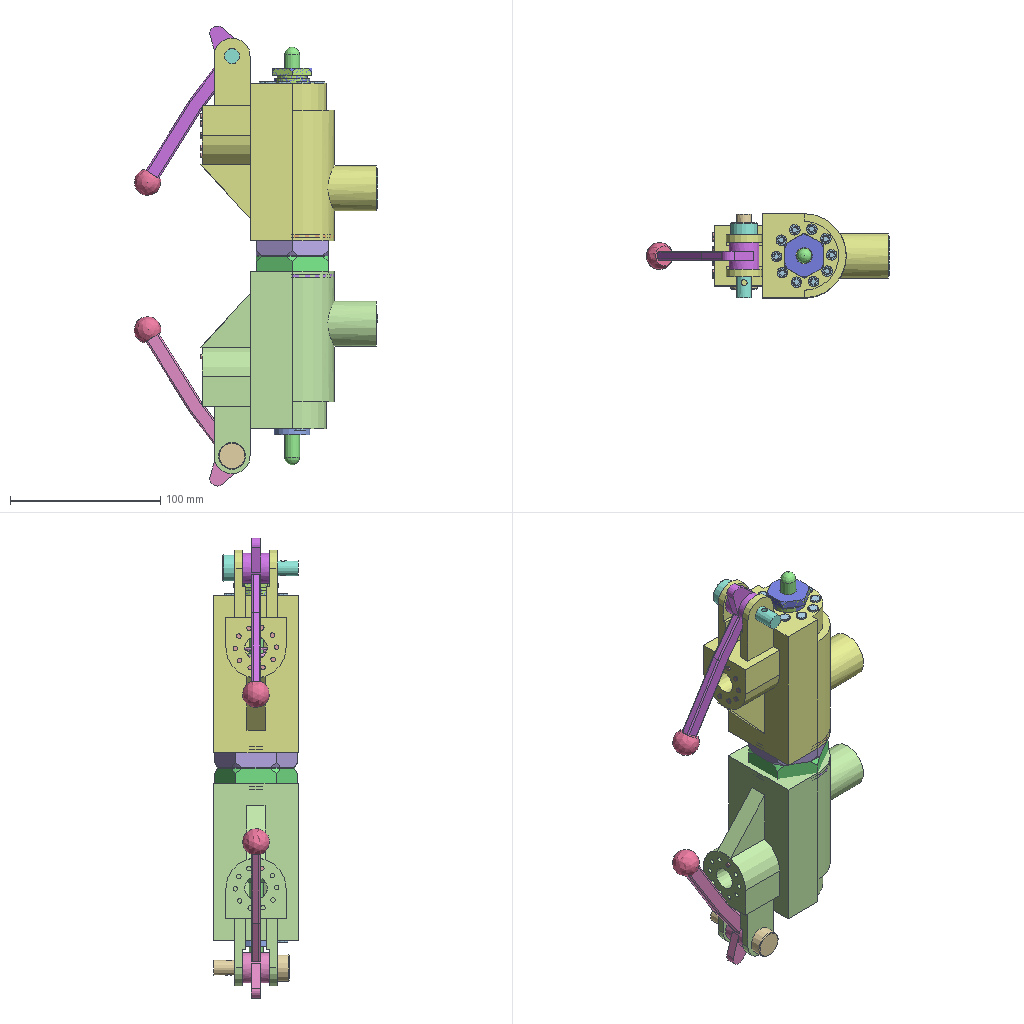Assembly | NX | 14 different items | 99 placed | box 162 x 56 x 306 mm
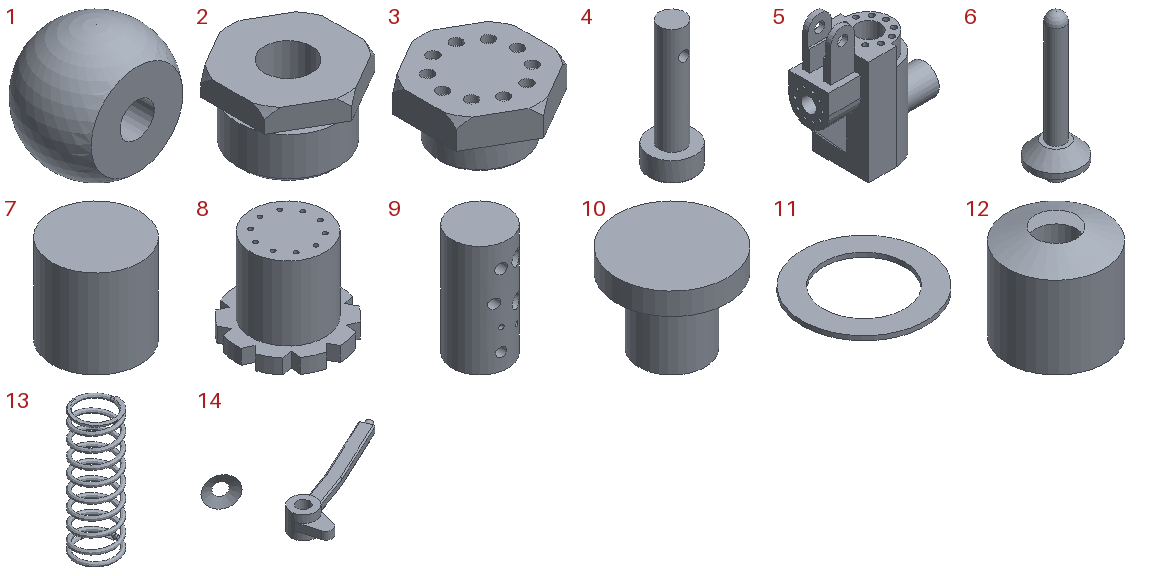Parts list (item | quantity | size | volume | features):
1 | x2 | 18 x 15 x 18 mm | 2621 mm3 | features ABSOLUTE_DATUM_PLANE 1, DATUM_CSYS 1, HOLE PACKAGE 1, SIMPLE HOLE 1, SPHERE 1, SYMBOLIC_THREAD 1, TRIM BODY 1
2 | x2 | - | 6271 mm3 | features CYLINDER 3, CHAMFER 2, DATUM_CSYS 2, EXTRUDE 2, INTERSECT 1, SKETCH 1, SYMBOLIC_THREAD 1
3 | x2 | - | 32370 mm3 | features CYLINDER 5, DATUM_CSYS 3, EXTRUDE 3, CHAMFER 2, SKETCH 2, INTERSECT 1, SYMBOLIC_THREAD 1
4 | x2 | 18 x 18 x 50 mm | 5204 mm3 | features CYLINDER 2, DATUM_CSYS 2, CHAMFER 1, EXTRUDE 1, SKETCH 1
5 | x2 | 116.842 x 56 x 135 mm | 278425 mm3 | features DATUM_CSYS 11, SKETCH 10, EXTRUDE 9, CYLINDER 8, BLEND 3, SYMBOLIC_THREAD 3, CHAMFER 2, CPROJ 2, UNITE 2, Container 1, EXTRACT_BODY 1, Geometry Instance 1, REPLACE_FACE 1
6 | x2 | 28 x 28 x 81 mm | 8685 mm3 | features CYLINDER 3, BLEND 1, CHAMFER 1, DATUM_CSYS 1, UNITE 1
7 | x20 | 3 x 3 x 3 mm | 21.206 mm3 | features CYLINDER 1, DATUM_CSYS 1
8 | x20 | 7 x 6.999 x 6 mm | 131.027 mm3 | features DATUM_CSYS 3, CYLINDER 2, EXTRUDE 2, SKETCH 2
9 | x20 | 3 x 3 x 6 mm | 37.933 mm3 | features DATUM_CSYS 2, CYLINDER 1, EXTRUDE 1, SKETCH 1
10 | x20 | 5 x 5 x 4 mm | 40.841 mm3 | features CYLINDER 2, DATUM_CSYS 1, UNITE 1
11 | x2 | 56 x 56 x 2 mm | 2776 mm3 | features DATUM_CSYS 2, SKETCH 1, SWP104 1
12 | x2 | 23.68 x 23.68 x 22.932 mm | 5989 mm3 | features DATUM_PLANE 2, EXTRUDE 2, DATUM_CSYS 1, LINKED_FACE 1, TRIM BODY 1
13 | x1 | - | 1950 mm3 | features SPLINE_LAW 3, BRIDGE_CURVE 2, DATUM_CSYS 2, DATUM_PLANE 2, TRIM BODY 2, ABSOLUTE_DATUM_AXIS 1, ABSOLUTE_DATUM_PLANE 1, DATUM_ON_PATH 1, FLEXIBLE_PART 1, FSET 1, SKETCH 1, SKIN 1
14 | x2 | 117.805 x 79.875 x 23.68 mm | 8790 mm3 | features DATUM_CSYS 4, EXTRUDE 3, SKETCH 3, CYLINDER 2, BLEND 1, CPROJ 1, LINKED_FACE 1
Mates (type | each side: item.copy, entity, surface, feature):
Touch | 13.1 plane | 3.1 face plane Cylinder(8)
Concentric | 11.1 edge | 3.1 edge
Touch | 6.1 face cylinder Cylinder(1) | 5.1 face cylinder Cylinder(19)
Touch | 6.1 face plane Cylinder(2) | 13.1 plane
Touch | 6.1 face cone Chamfer(3) | 5.1 face cone Chamfer(22)
Touch | 1.1 face cylinder Ø5 Hole(6) | 14.1 face cylinder Extrude(9)
Touch | 1.1 face plane Trim Body(5) | 14.1 face plane Extrude(2)
Concentric | 14.1 edge | 5.1 edge
Concentric | 4.1 edge | 5.1 edge
Concentric | 10.1 edge | 5.1 edge
Concentric | 7.1 edge | 3.1 edge
Concentric | 8.1 edge | 5.1 edge
Concentric | 9.1 edge | 5.1 edge